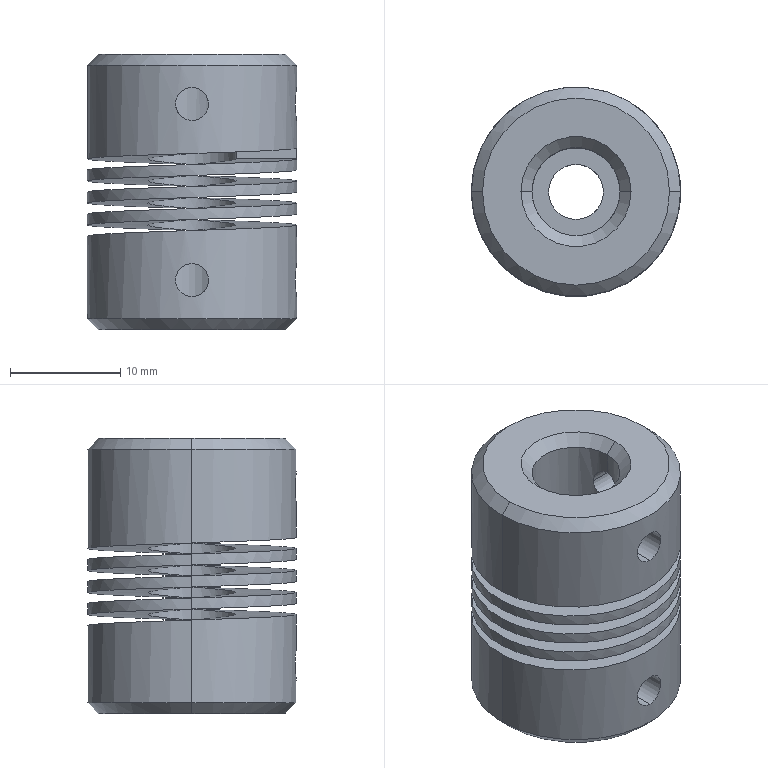Part | STEP file | 58 flexible coupling | 1 solid | 45 faces | box 19 x 19 x 25 mm | volume 4870 mm3 | cylinder 30 | cone 8 | plane 5 | spline 2 | commonest cylinder face diameters 8 x10 19 x10 3 x8 5 x2